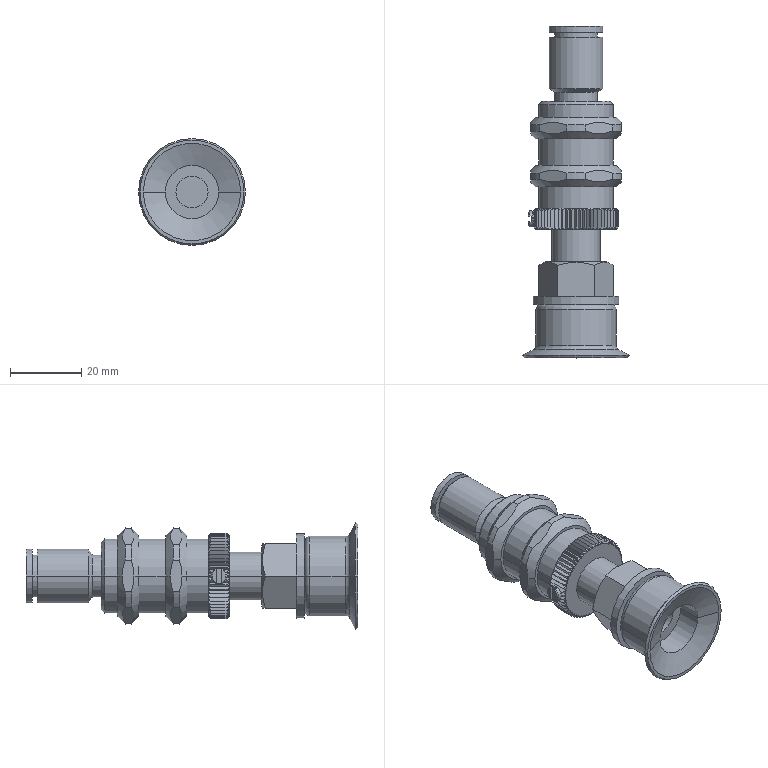Part | NX | 4 solids | 362 faces | box 30 x 93.15 x 30 mm | volume 27021 mm3 | plane 164 | cone 154 | cylinder 40 | torus 4 | commonest cylinder face diameters 27 x12 15 x6 9 x4 12 x4 17.753 x4 4.5 x2